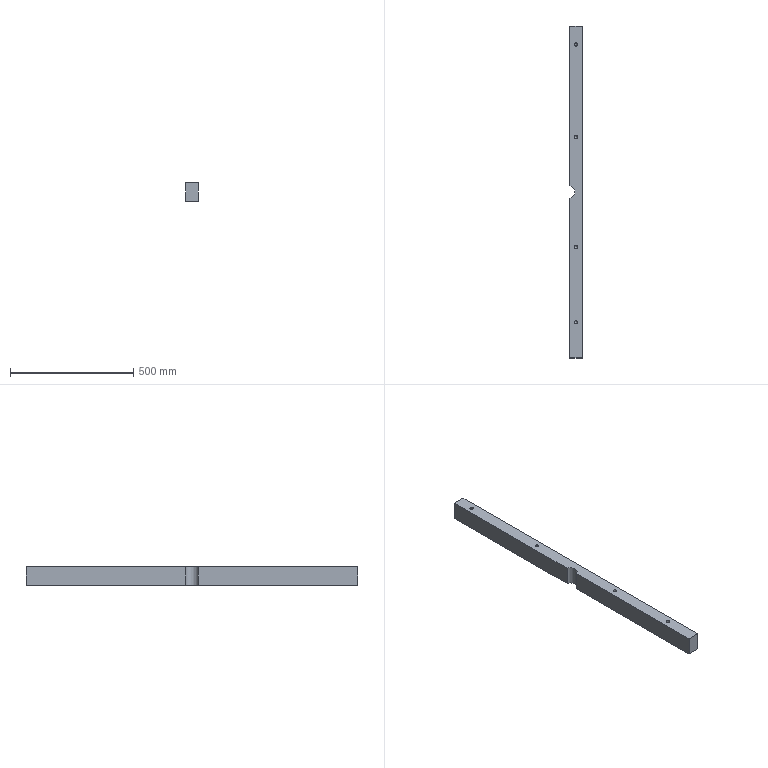Part | NX | features 3 2 | 1 solid | 24 faces | box 50 x 1345 x 75.5 mm | volume 5006269 mm3 | cylinder 9 | cone 8 | plane 7 | commonest cylinder face diameters 14.1 x8 54 x1
STEP:
#1=CARTESIAN_POINT('',(1789.05,-222.5,256.5));
#2=VERTEX_POINT('',#1);
#3=CARTESIAN_POINT('',(1782.,-222.5,256.5));
#4=DIRECTION('',(0.,0.,-1.));
#5=DIRECTION('',(1.,0.,0.));
#6=AXIS2_PLACEMENT_3D('',#3,#4,#5);
#7=CIRCLE('',#6,7.05);
#8=EDGE_CURVE('',#2,#2,#7,.T.);
#9=ORIENTED_EDGE('',*,*,#8,.T.);
#10=EDGE_LOOP('',(#9));
#11=FACE_BOUND('',#10,.T.);
#12=CARTESIAN_POINT('',(1789.05,222.5,256.5));
#13=VERTEX_POINT('',#12);
#14=CARTESIAN_POINT('',(1782.,222.5,256.5));
#15=DIRECTION('',(0.,0.,-1.));
#16=DIRECTION('',(1.,0.,0.));
#17=AXIS2_PLACEMENT_3D('',#14,#15,#16);
#18=CIRCLE('',#17,7.05);
#19=EDGE_CURVE('',#13,#13,#18,.T.);
#20=ORIENTED_EDGE('',*,*,#19,.T.);
#21=EDGE_LOOP('',(#20));
#22=FACE_BOUND('',#21,.T.);
#23=CARTESIAN_POINT('',(1757.,-26.077,256.5));
#24=VERTEX_POINT('',#23);
#25=CARTESIAN_POINT('',(1757.,26.077,256.5));
#26=VERTEX_POINT('',#25);
#27=CARTESIAN_POINT('',(1750.,0.,256.5));
#28=DIRECTION('',(0.,0.,1.));
#29=DIRECTION('',(1.,0.,0.));
#30=AXIS2_PLACEMENT_3D('',#27,#28,#29);
#31=CIRCLE('',#30,27.);
#32=EDGE_CURVE('',#24,#26,#31,.T.);
#33=ORIENTED_EDGE('',*,*,#32,.F.);
#34=CARTESIAN_POINT('',(1757.,-672.5,256.5));
#35=VERTEX_POINT('',#34);
#36=CARTESIAN_POINT('',(1757.,193.,256.5));
#37=DIRECTION('',(0.,1.,0.));
#38=VECTOR('',#37,1000.);
#39=LINE('',#36,#38);
#40=EDGE_CURVE('',#35,#24,#39,.T.);
#41=ORIENTED_EDGE('',*,*,#40,.F.);
#42=CARTESIAN_POINT('',(1807.,-672.5,256.5));
#43=VERTEX_POINT('',#42);
#44=CARTESIAN_POINT('',(3797.,-672.5,256.5));
#45=DIRECTION('',(1.,0.,0.));
#46=VECTOR('',#45,1000.);
#47=LINE('',#44,#46);
#48=EDGE_CURVE('',#35,#43,#47,.T.);
#49=ORIENTED_EDGE('',*,*,#48,.T.);
#50=CARTESIAN_POINT('',(1807.,672.5,256.5));
#51=VERTEX_POINT('',#50);
#52=CARTESIAN_POINT('',(1807.,193.,256.5));
#53=DIRECTION('',(0.,-1.,0.));
#54=VECTOR('',#53,1000.);
#55=LINE('',#52,#54);
#56=EDGE_CURVE('',#51,#43,#55,.T.);
#57=ORIENTED_EDGE('',*,*,#56,.F.);
#58=CARTESIAN_POINT('',(1757.,672.5,256.5));
#59=VERTEX_POINT('',#58);
#60=CARTESIAN_POINT('',(1757.,672.5,256.5));
#61=DIRECTION('',(1.,0.,0.));
#62=VECTOR('',#61,1000.);
#63=LINE('',#60,#62);
#64=EDGE_CURVE('',#59,#51,#63,.T.);
#65=ORIENTED_EDGE('',*,*,#64,.F.);
#66=CARTESIAN_POINT('',(1757.,193.,256.5));
#67=DIRECTION('',(0.,1.,0.));
#68=VECTOR('',#67,1000.);
#69=LINE('',#66,#68);
#70=EDGE_CURVE('',#26,#59,#69,.T.);
#71=ORIENTED_EDGE('',*,*,#70,.F.);
#72=EDGE_LOOP('',(#33,#41,#49,#57,#65,#71));
#73=FACE_BOUND('',#72,.T.);
#74=CARTESIAN_POINT('',(1789.05,597.5,256.5));
#75=VERTEX_POINT('',#74);
#76=CARTESIAN_POINT('',(1782.,597.5,256.5));
#77=DIRECTION('',(0.,0.,-1.));
#78=DIRECTION('',(1.,0.,0.));
#79=AXIS2_PLACEMENT_3D('',#76,#77,#78);
#80=CIRCLE('',#79,7.05);
#81=EDGE_CURVE('',#75,#75,#80,.T.);
#82=ORIENTED_EDGE('',*,*,#81,.T.);
#83=EDGE_LOOP('',(#82));
#84=FACE_BOUND('',#83,.T.);
#85=CARTESIAN_POINT('',(1789.05,-527.5,256.5));
#86=VERTEX_POINT('',#85);
#87=CARTESIAN_POINT('',(1782.,-527.5,256.5));
#88=DIRECTION('',(0.,0.,-1.));
#89=DIRECTION('',(1.,0.,0.));
#90=AXIS2_PLACEMENT_3D('',#87,#88,#89);
#91=CIRCLE('',#90,7.05);
#92=EDGE_CURVE('',#86,#86,#91,.T.);
#93=ORIENTED_EDGE('',*,*,#92,.T.);
#94=EDGE_LOOP('',(#93));
#95=FACE_BOUND('',#94,.T.);
#96=CARTESIAN_POINT('',(3797.,0.,256.5));
#97=DIRECTION('',(0.,0.,1.));
#98=DIRECTION('',(-1.,0.,0.));
#99=AXIS2_PLACEMENT_3D('',#96,#97,#98);
#100=PLANE('',#99);
#101=ADVANCED_FACE('',(#11,#22,#73,#84,#95),#100,.T.);
#102=CARTESIAN_POINT('',(1789.05,222.5,181.));
#103=VERTEX_POINT('',#102);
#104=CARTESIAN_POINT('',(1782.,222.5,181.));
#105=DIRECTION('',(0.,0.,1.));
#106=DIRECTION('',(1.,0.,0.));
#107=AXIS2_PLACEMENT_3D('',#104,#105,#106);
#108=CIRCLE('',#107,7.05);
#109=EDGE_CURVE('',#103,#103,#108,.T.);
#110=ORIENTED_EDGE('',*,*,#109,.T.);
#111=EDGE_LOOP('',(#110));
#112=FACE_BOUND('',#111,.T.);
#113=CARTESIAN_POINT('',(1789.05,-222.5,181.));
#114=VERTEX_POINT('',#113);
#115=CARTESIAN_POINT('',(1782.,-222.5,181.));
#116=DIRECTION('',(0.,0.,1.));
#117=DIRECTION('',(1.,0.,0.));
#118=AXIS2_PLACEMENT_3D('',#115,#116,#117);
#119=CIRCLE('',#118,7.05);
#120=EDGE_CURVE('',#114,#114,#119,.T.);
#121=ORIENTED_EDGE('',*,*,#120,.T.);
#122=EDGE_LOOP('',(#121));
#123=FACE_BOUND('',#122,.T.);
#124=CARTESIAN_POINT('',(1757.,26.077,181.));
#125=VERTEX_POINT('',#124);
#126=CARTESIAN_POINT('',(1757.,-26.077,181.));
#127=VERTEX_POINT('',#126);
#128=CARTESIAN_POINT('',(1750.,0.,181.));
#129=DIRECTION('',(0.,0.,-1.));
#130=DIRECTION('',(-1.,0.,0.));
#131=AXIS2_PLACEMENT_3D('',#128,#129,#130);
#132=CIRCLE('',#131,27.);
#133=EDGE_CURVE('',#125,#127,#132,.T.);
#134=ORIENTED_EDGE('',*,*,#133,.F.);
#135=CARTESIAN_POINT('',(1757.,672.5,181.));
#136=VERTEX_POINT('',#135);
#137=CARTESIAN_POINT('',(1757.,193.,181.));
#138=DIRECTION('',(0.,-1.,0.));
#139=VECTOR('',#138,1000.);
#140=LINE('',#137,#139);
#141=EDGE_CURVE('',#136,#125,#140,.T.);
#142=ORIENTED_EDGE('',*,*,#141,.F.);
#143=CARTESIAN_POINT('',(1807.,672.5,181.));
#144=VERTEX_POINT('',#143);
#145=CARTESIAN_POINT('',(3027.,672.5,181.));
#146=DIRECTION('',(1.,0.,0.));
#147=VECTOR('',#146,1000.);
#148=LINE('',#145,#147);
#149=EDGE_CURVE('',#136,#144,#148,.T.);
#150=ORIENTED_EDGE('',*,*,#149,.T.);
#151=CARTESIAN_POINT('',(1807.,-672.5,181.));
#152=VERTEX_POINT('',#151);
#153=CARTESIAN_POINT('',(1807.,193.,181.));
#154=DIRECTION('',(0.,1.,0.));
#155=VECTOR('',#154,1000.);
#156=LINE('',#153,#155);
#157=EDGE_CURVE('',#152,#144,#156,.T.);
#158=ORIENTED_EDGE('',*,*,#157,.F.);
#159=CARTESIAN_POINT('',(1757.,-672.5,181.));
#160=VERTEX_POINT('',#159);
#161=CARTESIAN_POINT('',(3027.,-672.5,181.));
#162=DIRECTION('',(-1.,0.,0.));
#163=VECTOR('',#162,1000.);
#164=LINE('',#161,#163);
#165=EDGE_CURVE('',#152,#160,#164,.T.);
#166=ORIENTED_EDGE('',*,*,#165,.T.);
#167=CARTESIAN_POINT('',(1757.,193.,181.));
#168=DIRECTION('',(0.,-1.,0.));
#169=VECTOR('',#168,1000.);
#170=LINE('',#167,#169);
#171=EDGE_CURVE('',#127,#160,#170,.T.);
#172=ORIENTED_EDGE('',*,*,#171,.F.);
#173=EDGE_LOOP('',(#134,#142,#150,#158,#166,#172));
#174=FACE_BOUND('',#173,.T.);
#175=CARTESIAN_POINT('',(1789.05,-527.5,181.));
#176=VERTEX_POINT('',#175);
#177=CARTESIAN_POINT('',(1782.,-527.5,181.));
#178=DIRECTION('',(0.,0.,1.));
#179=DIRECTION('',(1.,0.,0.));
#180=AXIS2_PLACEMENT_3D('',#177,#178,#179);
#181=CIRCLE('',#180,7.05);
#182=EDGE_CURVE('',#176,#176,#181,.T.);
#183=ORIENTED_EDGE('',*,*,#182,.T.);
#184=EDGE_LOOP('',(#183));
#185=FACE_BOUND('',#184,.T.);
#186=CARTESIAN_POINT('',(1789.05,597.5,181.));
#187=VERTEX_POINT('',#186);
#188=CARTESIAN_POINT('',(1782.,597.5,181.));
#189=DIRECTION('',(0.,0.,1.));
#190=DIRECTION('',(1.,0.,0.));
#191=AXIS2_PLACEMENT_3D('',#188,#189,#190);
#192=CIRCLE('',#191,7.05);
#193=EDGE_CURVE('',#187,#187,#192,.T.);
#194=ORIENTED_EDGE('',*,*,#193,.T.);
#195=EDGE_LOOP('',(#194));
#196=FACE_BOUND('',#195,.T.);
#197=CARTESIAN_POINT('',(3027.,193.,181.));
#198=DIRECTION('',(0.,0.,-1.));
#199=DIRECTION('',(-1.,0.,0.));
#200=AXIS2_PLACEMENT_3D('',#197,#198,#199);
#201=PLANE('',#200);
#202=ADVANCED_FACE('',(#112,#123,#174,#185,#196),#201,.T.);
#203=CARTESIAN_POINT('',(1757.,-26.077,-181.));
#204=DIRECTION('',(0.,0.,-1.));
#205=VECTOR('',#204,1000.);
#206=LINE('',#203,#205);
#207=EDGE_CURVE('',#24,#127,#206,.T.);
#208=ORIENTED_EDGE('',*,*,#207,.T.);
#209=ORIENTED_EDGE('',*,*,#171,.T.);
#210=CARTESIAN_POINT('',(1757.,-672.5,-1.5));
#211=DIRECTION('',(0.,0.,1.));
#212=VECTOR('',#211,1000.);
#213=LINE('',#210,#212);
#214=EDGE_CURVE('',#160,#35,#213,.T.);
#215=ORIENTED_EDGE('',*,*,#214,.T.);
#216=ORIENTED_EDGE('',*,*,#40,.T.);
#217=EDGE_LOOP('',(#208,#209,#215,#216));
#218=FACE_BOUND('',#217,.T.);
#219=CARTESIAN_POINT('',(1757.,193.,-1.5));
#220=DIRECTION('',(-1.,0.,0.));
#221=DIRECTION('',(0.,0.,-1.));
#222=AXIS2_PLACEMENT_3D('',#219,#220,#221);
#223=PLANE('',#222);
#224=ADVANCED_FACE('',(#218),#223,.T.);
#225=ORIENTED_EDGE('',*,*,#48,.F.);
#226=ORIENTED_EDGE('',*,*,#214,.F.);
#227=ORIENTED_EDGE('',*,*,#165,.F.);
#228=CARTESIAN_POINT('',(1807.,-672.5,-1.5));
#229=DIRECTION('',(0.,0.,-1.));
#230=VECTOR('',#229,1000.);
#231=LINE('',#228,#230);
#232=EDGE_CURVE('',#43,#152,#231,.T.);
#233=ORIENTED_EDGE('',*,*,#232,.F.);
#234=EDGE_LOOP('',(#225,#226,#227,#233));
#235=FACE_BOUND('',#234,.T.);
#236=CARTESIAN_POINT('',(284.5,-672.5,-103.));
#237=DIRECTION('',(0.,1.,0.));
#238=DIRECTION('',(1.,0.,0.));
#239=AXIS2_PLACEMENT_3D('',#236,#237,#238);
#240=PLANE('',#239);
#241=ADVANCED_FACE('',(#235),#240,.F.);
#242=CARTESIAN_POINT('',(1757.,26.077,181.));
#243=DIRECTION('',(0.,0.,1.));
#244=VECTOR('',#243,1000.);
#245=LINE('',#242,#244);
#246=EDGE_CURVE('',#125,#26,#245,.T.);
#247=ORIENTED_EDGE('',*,*,#246,.T.);
#248=ORIENTED_EDGE('',*,*,#70,.T.);
#249=CARTESIAN_POINT('',(1757.,672.5,-1.5));
#250=DIRECTION('',(0.,0.,-1.));
#251=VECTOR('',#250,1000.);
#252=LINE('',#249,#251);
#253=EDGE_CURVE('',#59,#136,#252,.T.);
#254=ORIENTED_EDGE('',*,*,#253,.T.);
#255=ORIENTED_EDGE('',*,*,#141,.T.);
#256=EDGE_LOOP('',(#247,#248,#254,#255));
#257=FACE_BOUND('',#256,.T.);
#258=CARTESIAN_POINT('',(1757.,193.,-1.5));
#259=DIRECTION('',(-1.,0.,0.));
#260=DIRECTION('',(0.,0.,-1.));
#261=AXIS2_PLACEMENT_3D('',#258,#259,#260);
#262=PLANE('',#261);
#263=ADVANCED_FACE('',(#257),#262,.T.);
#264=ORIENTED_EDGE('',*,*,#56,.T.);
#265=ORIENTED_EDGE('',*,*,#232,.T.);
#266=ORIENTED_EDGE('',*,*,#157,.T.);
#267=CARTESIAN_POINT('',(1807.,672.5,-1.5));
#268=DIRECTION('',(0.,0.,1.));
#269=VECTOR('',#268,1000.);
#270=LINE('',#267,#269);
#271=EDGE_CURVE('',#144,#51,#270,.T.);
#272=ORIENTED_EDGE('',*,*,#271,.T.);
#273=EDGE_LOOP('',(#264,#265,#266,#272));
#274=FACE_BOUND('',#273,.T.);
#275=CARTESIAN_POINT('',(1807.,193.,-1.5));
#276=DIRECTION('',(1.,0.,0.));
#277=DIRECTION('',(0.,0.,1.));
#278=AXIS2_PLACEMENT_3D('',#275,#276,#277);
#279=PLANE('',#278);
#280=ADVANCED_FACE('',(#274),#279,.T.);
#281=ORIENTED_EDGE('',*,*,#253,.F.);
#282=ORIENTED_EDGE('',*,*,#64,.T.);
#283=ORIENTED_EDGE('',*,*,#271,.F.);
#284=ORIENTED_EDGE('',*,*,#149,.F.);
#285=EDGE_LOOP('',(#281,#282,#283,#284));
#286=FACE_BOUND('',#285,.T.);
#287=CARTESIAN_POINT('',(1757.,672.5,231.5));
#288=DIRECTION('',(0.,1.,0.));
#289=DIRECTION('',(0.,0.,-1.));
#290=AXIS2_PLACEMENT_3D('',#287,#288,#289);
#291=PLANE('',#290);
#292=ADVANCED_FACE('',(#286),#291,.T.);
#293=ORIENTED_EDGE('',*,*,#32,.T.);
#294=ORIENTED_EDGE('',*,*,#246,.F.);
#295=ORIENTED_EDGE('',*,*,#133,.T.);
#296=ORIENTED_EDGE('',*,*,#207,.F.);
#297=EDGE_LOOP('',(#293,#294,#295,#296));
#298=FACE_BOUND('',#297,.T.);
#299=CARTESIAN_POINT('',(1750.,0.,-181.));
#300=DIRECTION('',(0.,0.,1.));
#301=DIRECTION('',(-1.,0.,0.));
#302=AXIS2_PLACEMENT_3D('',#299,#300,#301);
#303=CYLINDRICAL_SURFACE('',#302,27.);
#304=ADVANCED_FACE('',(#298),#303,.F.);
#305=CARTESIAN_POINT('',(1789.05,-222.5,188.95));
#306=VERTEX_POINT('',#305);
#307=CARTESIAN_POINT('',(1782.,-222.5,188.95));
#308=DIRECTION('',(0.,0.,1.));
#309=DIRECTION('',(1.,0.,0.));
#310=AXIS2_PLACEMENT_3D('',#307,#308,#309);
#311=CIRCLE('',#310,7.05);
#312=EDGE_CURVE('',#306,#306,#311,.T.);
#313=ORIENTED_EDGE('',*,*,#312,.T.);
#314=EDGE_LOOP('',(#313));
#315=FACE_BOUND('',#314,.T.);
#316=ORIENTED_EDGE('',*,*,#120,.F.);
#317=EDGE_LOOP('',(#316));
#318=FACE_BOUND('',#317,.T.);
#319=CARTESIAN_POINT('',(1782.,-222.5,181.));
#320=DIRECTION('',(0.,0.,1.));
#321=DIRECTION('',(-1.,0.,0.));
#322=AXIS2_PLACEMENT_3D('',#319,#320,#321);
#323=CYLINDRICAL_SURFACE('',#322,7.05);
#324=ADVANCED_FACE('',(#315,#318),#323,.F.);
#325=CARTESIAN_POINT('',(1782.,-222.5,196.));
#326=VERTEX_POINT('',#325);
#327=VERTEX_LOOP('',#326);
#328=FACE_BOUND('',#327,.T.);
#329=ORIENTED_EDGE('',*,*,#312,.F.);
#330=EDGE_LOOP('',(#329));
#331=FACE_BOUND('',#330,.T.);
#332=CARTESIAN_POINT('',(1782.,-222.5,188.95));
#333=DIRECTION('',(0.,0.,-1.));
#334=DIRECTION('',(1.,0.,0.));
#335=AXIS2_PLACEMENT_3D('',#332,#333,#334);
#336=CONICAL_SURFACE('',#335,7.05,0.7854);
#337=ADVANCED_FACE('',(#328,#331),#336,.F.);
#338=CARTESIAN_POINT('',(1789.05,-527.5,188.95));
#339=VERTEX_POINT('',#338);
#340=CARTESIAN_POINT('',(1782.,-527.5,188.95));
#341=DIRECTION('',(0.,0.,1.));
#342=DIRECTION('',(1.,0.,0.));
#343=AXIS2_PLACEMENT_3D('',#340,#341,#342);
#344=CIRCLE('',#343,7.05);
#345=EDGE_CURVE('',#339,#339,#344,.T.);
#346=ORIENTED_EDGE('',*,*,#345,.T.);
#347=EDGE_LOOP('',(#346));
#348=FACE_BOUND('',#347,.T.);
#349=ORIENTED_EDGE('',*,*,#182,.F.);
#350=EDGE_LOOP('',(#349));
#351=FACE_BOUND('',#350,.T.);
#352=CARTESIAN_POINT('',(1782.,-527.5,181.));
#353=DIRECTION('',(0.,0.,1.));
#354=DIRECTION('',(-1.,0.,0.));
#355=AXIS2_PLACEMENT_3D('',#352,#353,#354);
#356=CYLINDRICAL_SURFACE('',#355,7.05);
#357=ADVANCED_FACE('',(#348,#351),#356,.F.);
#358=CARTESIAN_POINT('',(1782.,-527.5,196.));
#359=VERTEX_POINT('',#358);
#360=VERTEX_LOOP('',#359);
#361=FACE_BOUND('',#360,.T.);
#362=ORIENTED_EDGE('',*,*,#345,.F.);
#363=EDGE_LOOP('',(#362));
#364=FACE_BOUND('',#363,.T.);
#365=CARTESIAN_POINT('',(1782.,-527.5,188.95));
#366=DIRECTION('',(0.,0.,-1.));
#367=DIRECTION('',(1.,0.,0.));
#368=AXIS2_PLACEMENT_3D('',#365,#366,#367);
#369=CONICAL_SURFACE('',#368,7.05,0.7854);
#370=ADVANCED_FACE('',(#361,#364),#369,.F.);
#371=CARTESIAN_POINT('',(1789.05,222.5,188.95));
#372=VERTEX_POINT('',#371);
#373=CARTESIAN_POINT('',(1782.,222.5,188.95));
#374=DIRECTION('',(0.,0.,1.));
#375=DIRECTION('',(1.,0.,0.));
#376=AXIS2_PLACEMENT_3D('',#373,#374,#375);
#377=CIRCLE('',#376,7.05);
#378=EDGE_CURVE('',#372,#372,#377,.T.);
#379=ORIENTED_EDGE('',*,*,#378,.T.);
#380=EDGE_LOOP('',(#379));
#381=FACE_BOUND('',#380,.T.);
#382=ORIENTED_EDGE('',*,*,#109,.F.);
#383=EDGE_LOOP('',(#382));
#384=FACE_BOUND('',#383,.T.);
#385=CARTESIAN_POINT('',(1782.,222.5,181.));
#386=DIRECTION('',(0.,0.,1.));
#387=DIRECTION('',(-1.,0.,0.));
#388=AXIS2_PLACEMENT_3D('',#385,#386,#387);
#389=CYLINDRICAL_SURFACE('',#388,7.05);
#390=ADVANCED_FACE('',(#381,#384),#389,.F.);
#391=CARTESIAN_POINT('',(1782.,222.5,196.));
#392=VERTEX_POINT('',#391);
#393=VERTEX_LOOP('',#392);
#394=FACE_BOUND('',#393,.T.);
#395=ORIENTED_EDGE('',*,*,#378,.F.);
#396=EDGE_LOOP('',(#395));
#397=FACE_BOUND('',#396,.T.);
#398=CARTESIAN_POINT('',(1782.,222.5,188.95));
#399=DIRECTION('',(0.,0.,-1.));
#400=DIRECTION('',(1.,0.,0.));
#401=AXIS2_PLACEMENT_3D('',#398,#399,#400);
#402=CONICAL_SURFACE('',#401,7.05,0.7854);
#403=ADVANCED_FACE('',(#394,#397),#402,.F.);
#404=CARTESIAN_POINT('',(1789.05,597.5,188.95));
#405=VERTEX_POINT('',#404);
#406=CARTESIAN_POINT('',(1782.,597.5,188.95));
#407=DIRECTION('',(0.,0.,1.));
#408=DIRECTION('',(1.,0.,0.));
#409=AXIS2_PLACEMENT_3D('',#406,#407,#408);
#410=CIRCLE('',#409,7.05);
#411=EDGE_CURVE('',#405,#405,#410,.T.);
#412=ORIENTED_EDGE('',*,*,#411,.T.);
#413=EDGE_LOOP('',(#412));
#414=FACE_BOUND('',#413,.T.);
#415=ORIENTED_EDGE('',*,*,#193,.F.);
#416=EDGE_LOOP('',(#415));
#417=FACE_BOUND('',#416,.T.);
#418=CARTESIAN_POINT('',(1782.,597.5,181.));
#419=DIRECTION('',(0.,0.,1.));
#420=DIRECTION('',(-1.,0.,0.));
#421=AXIS2_PLACEMENT_3D('',#418,#419,#420);
#422=CYLINDRICAL_SURFACE('',#421,7.05);
#423=ADVANCED_FACE('',(#414,#417),#422,.F.);
#424=CARTESIAN_POINT('',(1782.,597.5,196.));
#425=VERTEX_POINT('',#424);
#426=VERTEX_LOOP('',#425);
#427=FACE_BOUND('',#426,.T.);
#428=ORIENTED_EDGE('',*,*,#411,.F.);
#429=EDGE_LOOP('',(#428));
#430=FACE_BOUND('',#429,.T.);
#431=CARTESIAN_POINT('',(1782.,597.5,188.95));
#432=DIRECTION('',(0.,0.,-1.));
#433=DIRECTION('',(1.,0.,0.));
#434=AXIS2_PLACEMENT_3D('',#431,#432,#433);
#435=CONICAL_SURFACE('',#434,7.05,0.7854);
#436=ADVANCED_FACE('',(#427,#430),#435,.F.);
#437=CARTESIAN_POINT('',(1774.95,222.5,248.55));
#438=VERTEX_POINT('',#437);
#439=CARTESIAN_POINT('',(1782.,222.5,248.55));
#440=DIRECTION('',(0.,0.,-1.));
#441=DIRECTION('',(-1.,0.,0.));
#442=AXIS2_PLACEMENT_3D('',#439,#440,#441);
#443=CIRCLE('',#442,7.05);
#444=EDGE_CURVE('',#438,#438,#443,.T.);
#445=ORIENTED_EDGE('',*,*,#444,.T.);
#446=EDGE_LOOP('',(#445));
#447=FACE_BOUND('',#446,.T.);
#448=ORIENTED_EDGE('',*,*,#19,.F.);
#449=EDGE_LOOP('',(#448));
#450=FACE_BOUND('',#449,.T.);
#451=CARTESIAN_POINT('',(1782.,222.5,256.5));
#452=DIRECTION('',(0.,0.,-1.));
#453=DIRECTION('',(-1.,0.,0.));
#454=AXIS2_PLACEMENT_3D('',#451,#452,#453);
#455=CYLINDRICAL_SURFACE('',#454,7.05);
#456=ADVANCED_FACE('',(#447,#450),#455,.F.);
#457=CARTESIAN_POINT('',(1782.,222.5,241.5));
#458=VERTEX_POINT('',#457);
#459=VERTEX_LOOP('',#458);
#460=FACE_BOUND('',#459,.T.);
#461=ORIENTED_EDGE('',*,*,#444,.F.);
#462=EDGE_LOOP('',(#461));
#463=FACE_BOUND('',#462,.T.);
#464=CARTESIAN_POINT('',(1782.,222.5,248.55));
#465=DIRECTION('',(0.,0.,1.));
#466=DIRECTION('',(-1.,0.,0.));
#467=AXIS2_PLACEMENT_3D('',#464,#465,#466);
#468=CONICAL_SURFACE('',#467,7.05,0.7854);
#469=ADVANCED_FACE('',(#460,#463),#468,.F.);
#470=CARTESIAN_POINT('',(1774.95,597.5,248.55));
#471=VERTEX_POINT('',#470);
#472=CARTESIAN_POINT('',(1782.,597.5,248.55));
#473=DIRECTION('',(0.,0.,-1.));
#474=DIRECTION('',(-1.,0.,0.));
#475=AXIS2_PLACEMENT_3D('',#472,#473,#474);
#476=CIRCLE('',#475,7.05);
#477=EDGE_CURVE('',#471,#471,#476,.T.);
#478=ORIENTED_EDGE('',*,*,#477,.T.);
#479=EDGE_LOOP('',(#478));
#480=FACE_BOUND('',#479,.T.);
#481=ORIENTED_EDGE('',*,*,#81,.F.);
#482=EDGE_LOOP('',(#481));
#483=FACE_BOUND('',#482,.T.);
#484=CARTESIAN_POINT('',(1782.,597.5,256.5));
#485=DIRECTION('',(0.,0.,-1.));
#486=DIRECTION('',(-1.,0.,0.));
#487=AXIS2_PLACEMENT_3D('',#484,#485,#486);
#488=CYLINDRICAL_SURFACE('',#487,7.05);
#489=ADVANCED_FACE('',(#480,#483),#488,.F.);
#490=CARTESIAN_POINT('',(1782.,597.5,241.5));
#491=VERTEX_POINT('',#490);
#492=VERTEX_LOOP('',#491);
#493=FACE_BOUND('',#492,.T.);
#494=ORIENTED_EDGE('',*,*,#477,.F.);
#495=EDGE_LOOP('',(#494));
#496=FACE_BOUND('',#495,.T.);
#497=CARTESIAN_POINT('',(1782.,597.5,248.55));
#498=DIRECTION('',(0.,0.,1.));
#499=DIRECTION('',(-1.,0.,0.));
#500=AXIS2_PLACEMENT_3D('',#497,#498,#499);
#501=CONICAL_SURFACE('',#500,7.05,0.7854);
#502=ADVANCED_FACE('',(#493,#496),#501,.F.);
#503=CARTESIAN_POINT('',(1774.95,-222.5,248.55));
#504=VERTEX_POINT('',#503);
#505=CARTESIAN_POINT('',(1782.,-222.5,248.55));
#506=DIRECTION('',(0.,0.,-1.));
#507=DIRECTION('',(-1.,0.,0.));
#508=AXIS2_PLACEMENT_3D('',#505,#506,#507);
#509=CIRCLE('',#508,7.05);
#510=EDGE_CURVE('',#504,#504,#509,.T.);
#511=ORIENTED_EDGE('',*,*,#510,.T.);
#512=EDGE_LOOP('',(#511));
#513=FACE_BOUND('',#512,.T.);
#514=ORIENTED_EDGE('',*,*,#8,.F.);
#515=EDGE_LOOP('',(#514));
#516=FACE_BOUND('',#515,.T.);
#517=CARTESIAN_POINT('',(1782.,-222.5,256.5));
#518=DIRECTION('',(0.,0.,-1.));
#519=DIRECTION('',(-1.,0.,0.));
#520=AXIS2_PLACEMENT_3D('',#517,#518,#519);
#521=CYLINDRICAL_SURFACE('',#520,7.05);
#522=ADVANCED_FACE('',(#513,#516),#521,.F.);
#523=CARTESIAN_POINT('',(1782.,-222.5,241.5));
#524=VERTEX_POINT('',#523);
#525=VERTEX_LOOP('',#524);
#526=FACE_BOUND('',#525,.T.);
#527=ORIENTED_EDGE('',*,*,#510,.F.);
#528=EDGE_LOOP('',(#527));
#529=FACE_BOUND('',#528,.T.);
#530=CARTESIAN_POINT('',(1782.,-222.5,248.55));
#531=DIRECTION('',(0.,0.,1.));
#532=DIRECTION('',(-1.,0.,0.));
#533=AXIS2_PLACEMENT_3D('',#530,#531,#532);
#534=CONICAL_SURFACE('',#533,7.05,0.7854);
#535=ADVANCED_FACE('',(#526,#529),#534,.F.);
#536=CARTESIAN_POINT('',(1774.95,-527.5,248.55));
#537=VERTEX_POINT('',#536);
#538=CARTESIAN_POINT('',(1782.,-527.5,248.55));
#539=DIRECTION('',(0.,0.,-1.));
#540=DIRECTION('',(-1.,0.,0.));
#541=AXIS2_PLACEMENT_3D('',#538,#539,#540);
#542=CIRCLE('',#541,7.05);
#543=EDGE_CURVE('',#537,#537,#542,.T.);
#544=ORIENTED_EDGE('',*,*,#543,.T.);
#545=EDGE_LOOP('',(#544));
#546=FACE_BOUND('',#545,.T.);
#547=ORIENTED_EDGE('',*,*,#92,.F.);
#548=EDGE_LOOP('',(#547));
#549=FACE_BOUND('',#548,.T.);
#550=CARTESIAN_POINT('',(1782.,-527.5,256.5));
#551=DIRECTION('',(0.,0.,-1.));
#552=DIRECTION('',(-1.,0.,0.));
#553=AXIS2_PLACEMENT_3D('',#550,#551,#552);
#554=CYLINDRICAL_SURFACE('',#553,7.05);
#555=ADVANCED_FACE('',(#546,#549),#554,.F.);
#556=CARTESIAN_POINT('',(1782.,-527.5,241.5));
#557=VERTEX_POINT('',#556);
#558=VERTEX_LOOP('',#557);
#559=FACE_BOUND('',#558,.T.);
#560=ORIENTED_EDGE('',*,*,#543,.F.);
#561=EDGE_LOOP('',(#560));
#562=FACE_BOUND('',#561,.T.);
#563=CARTESIAN_POINT('',(1782.,-527.5,248.55));
#564=DIRECTION('',(0.,0.,1.));
#565=DIRECTION('',(-1.,0.,0.));
#566=AXIS2_PLACEMENT_3D('',#563,#564,#565);
#567=CONICAL_SURFACE('',#566,7.05,0.7854);
#568=ADVANCED_FACE('',(#559,#562),#567,.F.);
#569=CLOSED_SHELL('',(#101,#202,#224,#241,#263,#280,#292,#304,#324,#337,#357,#370,#390,#403,#423,#436,#456,#469,#489,#502,#522,#535,#555,#568));
#570=MANIFOLD_SOLID_BREP('',#569);
#571=(LENGTH_UNIT()NAMED_UNIT(*)SI_UNIT(.MILLI.,.METRE.));
#572=UNCERTAINTY_MEASURE_WITH_UNIT(LENGTH_MEASURE(0.00001),#571,'','');
#573=(NAMED_UNIT(*)PLANE_ANGLE_UNIT()SI_UNIT($,.RADIAN.));
#574=(NAMED_UNIT(*)SI_UNIT($,.STERADIAN.)SOLID_ANGLE_UNIT());
#575=(GEOMETRIC_REPRESENTATION_CONTEXT(3)GLOBAL_UNCERTAINTY_ASSIGNED_CONTEXT((#572))GLOBAL_UNIT_ASSIGNED_CONTEXT((#571,#573,#574))REPRESENTATION_CONTEXT('',''));
#576=ADVANCED_BREP_SHAPE_REPRESENTATION('',(#570),#575);